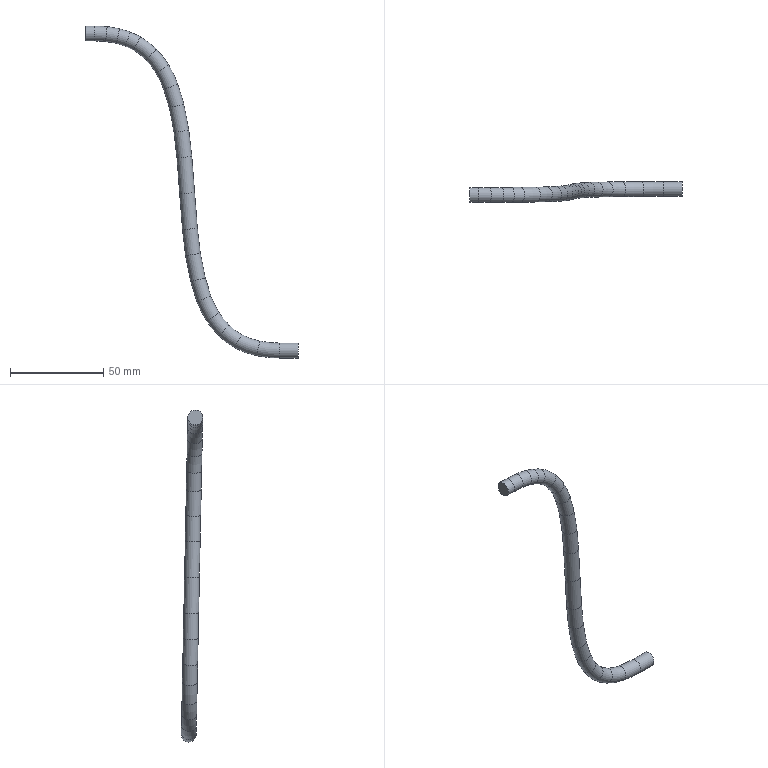Part | STEP file | solid 136 | 1 solid | 24 faces | box 113.804 x 11.5 x 178 mm | volume 11895 mm3 | torus 20 | cylinder 2 | plane 2 | commonest cylinder face diameters 8 x2